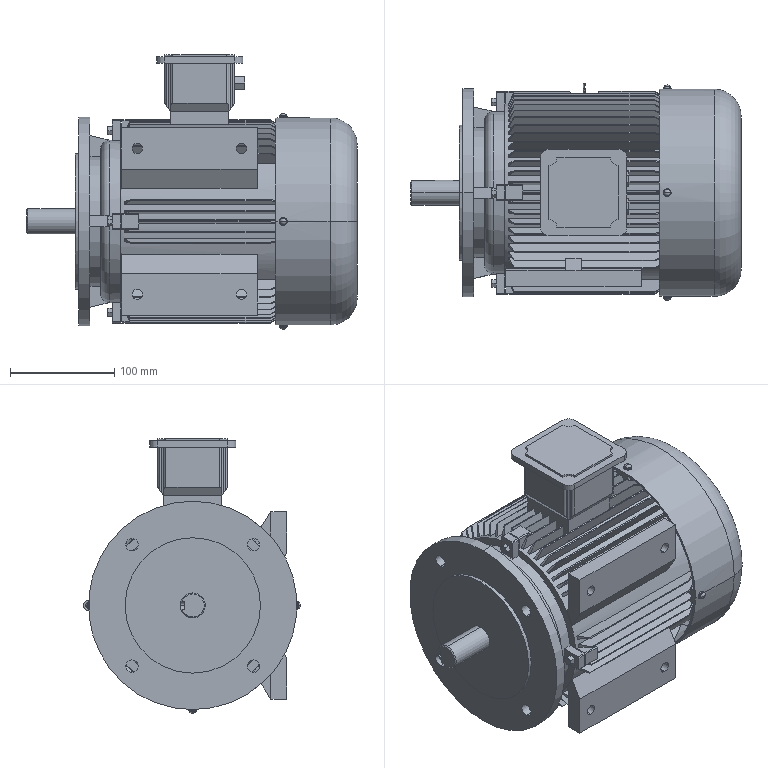Part | SolidWorks | features Boss 18, Cut 6, Revolution 5, CirPattern 4, Fillet 4, Chamfer 3, RevCut 2, 3DProfileFeature 1, LPattern 1, MirrorPattern 1, MoveCopyBody 1 | 2 solids | 660 faces | box 317 x 208.5 x 263.5 mm | volume 6287758 mm3 | plane 405 | cone 134 | cylinder 99 | torus 14 | sphere 8 | commonest cylinder face diameters 3.937 x10 171 x10 5.5 x9 6.7 x8 7.5 x8 10 x8